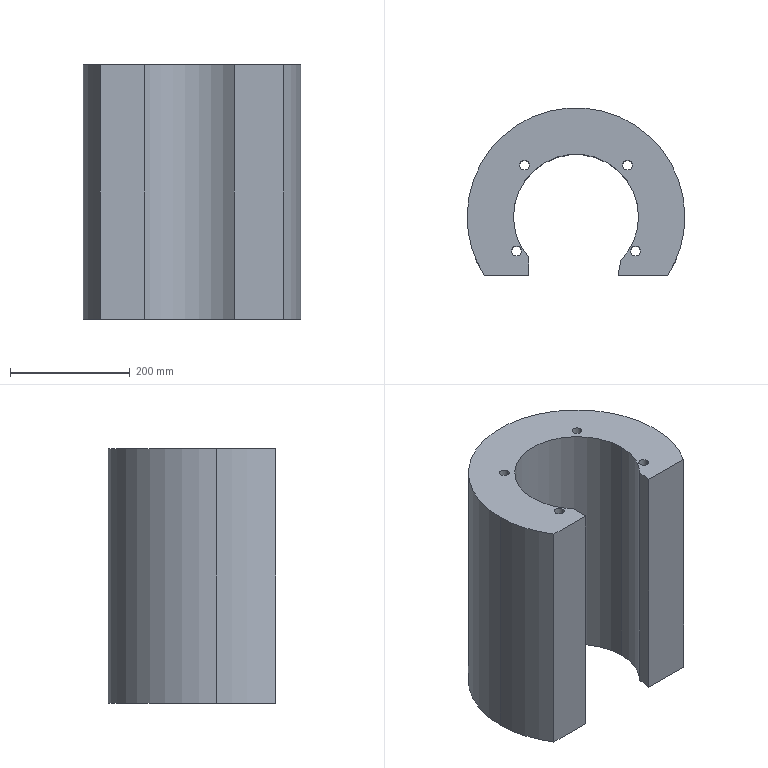Part | SolidWorks | features Extrusion 1 | 1 solid | 20 faces | box 364.306 x 280.408 x 426 mm | volume 21434816 mm3 | cylinder 14 | plane 6 | commonest cylinder face diameters 16 x4 16.5 x4 209.233 x3 364.306 x3
STEP:
#1=CARTESIAN_POINT('',(-19.917,-80.848,-426.));
#2=VERTEX_POINT('',#1);
#3=CARTESIAN_POINT('',(-3.417,-80.848,-426.));
#4=VERTEX_POINT('',#3);
#5=CARTESIAN_POINT('',(-11.667,-80.848,-426.));
#6=DIRECTION('',(0.,0.,1.));
#7=DIRECTION('',(1.,0.,0.));
#8=AXIS2_PLACEMENT_3D('',#5,#6,#7);
#9=CIRCLE('',#8,8.25);
#10=EDGE_CURVE('',#2,#4,#9,.T.);
#11=ORIENTED_EDGE('',*,*,#10,.F.);
#12=CARTESIAN_POINT('',(-19.917,-80.848,0.));
#13=VERTEX_POINT('',#12);
#14=CARTESIAN_POINT('',(-19.917,-80.848,-426.));
#15=DIRECTION('',(0.,0.,1.));
#16=VECTOR('',#15,1000.);
#17=LINE('',#14,#16);
#18=EDGE_CURVE('',#2,#13,#17,.T.);
#19=ORIENTED_EDGE('',*,*,#18,.T.);
#20=CARTESIAN_POINT('',(-3.417,-80.848,0.));
#21=VERTEX_POINT('',#20);
#22=CARTESIAN_POINT('',(-11.667,-80.848,0.));
#23=DIRECTION('',(0.,0.,1.));
#24=DIRECTION('',(1.,0.,0.));
#25=AXIS2_PLACEMENT_3D('',#22,#23,#24);
#26=CIRCLE('',#25,8.25);
#27=EDGE_CURVE('',#13,#21,#26,.T.);
#28=ORIENTED_EDGE('',*,*,#27,.T.);
#29=CARTESIAN_POINT('',(-3.417,-80.848,-426.));
#30=DIRECTION('',(0.,0.,1.));
#31=VECTOR('',#30,1000.);
#32=LINE('',#29,#31);
#33=EDGE_CURVE('',#4,#21,#32,.T.);
#34=ORIENTED_EDGE('',*,*,#33,.F.);
#35=EDGE_LOOP('',(#11,#19,#28,#34));
#36=FACE_OUTER_BOUND('',#35,.T.);
#37=CARTESIAN_POINT('',(-11.667,-80.848,-426.));
#38=DIRECTION('',(0.,0.,1.));
#39=DIRECTION('',(1.,0.,0.));
#40=AXIS2_PLACEMENT_3D('',#37,#38,#39);
#41=CYLINDRICAL_SURFACE('',#40,8.25);
#42=ADVANCED_FACE('',(#36),#41,.F.);
#43=CARTESIAN_POINT('',(-219.103,-80.848,-426.));
#44=VERTEX_POINT('',#43);
#45=CARTESIAN_POINT('',(-202.603,-80.848,-426.));
#46=VERTEX_POINT('',#45);
#47=CARTESIAN_POINT('',(-210.853,-80.848,-426.));
#48=DIRECTION('',(0.,0.,1.));
#49=DIRECTION('',(1.,0.,0.));
#50=AXIS2_PLACEMENT_3D('',#47,#48,#49);
#51=CIRCLE('',#50,8.25);
#52=EDGE_CURVE('',#44,#46,#51,.T.);
#53=ORIENTED_EDGE('',*,*,#52,.F.);
#54=CARTESIAN_POINT('',(-219.103,-80.848,0.));
#55=VERTEX_POINT('',#54);
#56=CARTESIAN_POINT('',(-219.103,-80.848,-426.));
#57=DIRECTION('',(0.,0.,1.));
#58=VECTOR('',#57,1000.);
#59=LINE('',#56,#58);
#60=EDGE_CURVE('',#44,#55,#59,.T.);
#61=ORIENTED_EDGE('',*,*,#60,.T.);
#62=CARTESIAN_POINT('',(-202.603,-80.848,0.));
#63=VERTEX_POINT('',#62);
#64=CARTESIAN_POINT('',(-210.853,-80.848,0.));
#65=DIRECTION('',(0.,0.,1.));
#66=DIRECTION('',(1.,0.,0.));
#67=AXIS2_PLACEMENT_3D('',#64,#65,#66);
#68=CIRCLE('',#67,8.25);
#69=EDGE_CURVE('',#55,#63,#68,.T.);
#70=ORIENTED_EDGE('',*,*,#69,.T.);
#71=CARTESIAN_POINT('',(-202.603,-80.848,-426.));
#72=DIRECTION('',(0.,0.,1.));
#73=VECTOR('',#72,1000.);
#74=LINE('',#71,#73);
#75=EDGE_CURVE('',#46,#63,#74,.T.);
#76=ORIENTED_EDGE('',*,*,#75,.F.);
#77=EDGE_LOOP('',(#53,#61,#70,#76));
#78=FACE_OUTER_BOUND('',#77,.T.);
#79=CARTESIAN_POINT('',(-210.853,-80.848,-426.));
#80=DIRECTION('',(0.,0.,1.));
#81=DIRECTION('',(1.,0.,0.));
#82=AXIS2_PLACEMENT_3D('',#79,#80,#81);
#83=CYLINDRICAL_SURFACE('',#82,8.25);
#84=ADVANCED_FACE('',(#78),#83,.F.);
#85=CARTESIAN_POINT('',(-205.527,62.919,-426.));
#86=VERTEX_POINT('',#85);
#87=CARTESIAN_POINT('',(-189.527,62.919,-426.));
#88=VERTEX_POINT('',#87);
#89=CARTESIAN_POINT('',(-197.527,62.919,-426.));
#90=DIRECTION('',(0.,0.,1.));
#91=DIRECTION('',(1.,0.,0.));
#92=AXIS2_PLACEMENT_3D('',#89,#90,#91);
#93=CIRCLE('',#92,8.);
#94=EDGE_CURVE('',#86,#88,#93,.T.);
#95=ORIENTED_EDGE('',*,*,#94,.F.);
#96=CARTESIAN_POINT('',(-205.527,62.919,0.));
#97=VERTEX_POINT('',#96);
#98=CARTESIAN_POINT('',(-205.527,62.919,-426.));
#99=DIRECTION('',(0.,0.,1.));
#100=VECTOR('',#99,1000.);
#101=LINE('',#98,#100);
#102=EDGE_CURVE('',#86,#97,#101,.T.);
#103=ORIENTED_EDGE('',*,*,#102,.T.);
#104=CARTESIAN_POINT('',(-189.527,62.919,0.));
#105=VERTEX_POINT('',#104);
#106=CARTESIAN_POINT('',(-197.527,62.919,0.));
#107=DIRECTION('',(0.,0.,1.));
#108=DIRECTION('',(1.,0.,0.));
#109=AXIS2_PLACEMENT_3D('',#106,#107,#108);
#110=CIRCLE('',#109,8.);
#111=EDGE_CURVE('',#97,#105,#110,.T.);
#112=ORIENTED_EDGE('',*,*,#111,.T.);
#113=CARTESIAN_POINT('',(-189.527,62.919,-426.));
#114=DIRECTION('',(0.,0.,1.));
#115=VECTOR('',#114,1000.);
#116=LINE('',#113,#115);
#117=EDGE_CURVE('',#88,#105,#116,.T.);
#118=ORIENTED_EDGE('',*,*,#117,.F.);
#119=EDGE_LOOP('',(#95,#103,#112,#118));
#120=FACE_OUTER_BOUND('',#119,.T.);
#121=CARTESIAN_POINT('',(-197.527,62.919,-426.));
#122=DIRECTION('',(0.,0.,1.));
#123=DIRECTION('',(1.,0.,0.));
#124=AXIS2_PLACEMENT_3D('',#121,#122,#123);
#125=CYLINDRICAL_SURFACE('',#124,8.);
#126=ADVANCED_FACE('',(#120),#125,.F.);
#127=CARTESIAN_POINT('',(-32.993,62.919,-426.));
#128=VERTEX_POINT('',#127);
#129=CARTESIAN_POINT('',(-16.993,62.919,-426.));
#130=VERTEX_POINT('',#129);
#131=CARTESIAN_POINT('',(-24.993,62.919,-426.));
#132=DIRECTION('',(0.,0.,1.));
#133=DIRECTION('',(1.,0.,0.));
#134=AXIS2_PLACEMENT_3D('',#131,#132,#133);
#135=CIRCLE('',#134,8.);
#136=EDGE_CURVE('',#128,#130,#135,.T.);
#137=ORIENTED_EDGE('',*,*,#136,.F.);
#138=CARTESIAN_POINT('',(-32.993,62.919,0.));
#139=VERTEX_POINT('',#138);
#140=CARTESIAN_POINT('',(-32.993,62.919,-426.));
#141=DIRECTION('',(0.,0.,1.));
#142=VECTOR('',#141,1000.);
#143=LINE('',#140,#142);
#144=EDGE_CURVE('',#128,#139,#143,.T.);
#145=ORIENTED_EDGE('',*,*,#144,.T.);
#146=CARTESIAN_POINT('',(-16.993,62.919,0.));
#147=VERTEX_POINT('',#146);
#148=CARTESIAN_POINT('',(-24.993,62.919,0.));
#149=DIRECTION('',(0.,0.,1.));
#150=DIRECTION('',(1.,0.,0.));
#151=AXIS2_PLACEMENT_3D('',#148,#149,#150);
#152=CIRCLE('',#151,8.);
#153=EDGE_CURVE('',#139,#147,#152,.T.);
#154=ORIENTED_EDGE('',*,*,#153,.T.);
#155=CARTESIAN_POINT('',(-16.993,62.919,-426.));
#156=DIRECTION('',(0.,0.,1.));
#157=VECTOR('',#156,1000.);
#158=LINE('',#155,#157);
#159=EDGE_CURVE('',#130,#147,#158,.T.);
#160=ORIENTED_EDGE('',*,*,#159,.F.);
#161=EDGE_LOOP('',(#137,#145,#154,#160));
#162=FACE_OUTER_BOUND('',#161,.T.);
#163=CARTESIAN_POINT('',(-24.993,62.919,-426.));
#164=DIRECTION('',(0.,0.,1.));
#165=DIRECTION('',(1.,0.,0.));
#166=AXIS2_PLACEMENT_3D('',#163,#164,#165);
#167=CYLINDRICAL_SURFACE('',#166,8.);
#168=ADVANCED_FACE('',(#162),#167,.F.);
#169=CARTESIAN_POINT('',(-189.998,-92.232,-426.));
#170=VERTEX_POINT('',#169);
#171=CARTESIAN_POINT('',(-215.877,-23.348,-426.));
#172=VERTEX_POINT('',#171);
#173=CARTESIAN_POINT('',(-111.26,-23.348,-426.));
#174=DIRECTION('',(0.,0.,-1.));
#175=DIRECTION('',(1.,0.,0.));
#176=AXIS2_PLACEMENT_3D('',#173,#174,#175);
#177=CIRCLE('',#176,104.617);
#178=EDGE_CURVE('',#170,#172,#177,.T.);
#179=ORIENTED_EDGE('',*,*,#178,.T.);
#180=CARTESIAN_POINT('',(-215.877,-23.348,0.));
#181=VERTEX_POINT('',#180);
#182=CARTESIAN_POINT('',(-215.877,-23.348,-426.));
#183=DIRECTION('',(0.,0.,1.));
#184=VECTOR('',#183,1000.);
#185=LINE('',#182,#184);
#186=EDGE_CURVE('',#172,#181,#185,.T.);
#187=ORIENTED_EDGE('',*,*,#186,.T.);
#188=CARTESIAN_POINT('',(-189.998,-92.232,0.));
#189=VERTEX_POINT('',#188);
#190=CARTESIAN_POINT('',(-111.26,-23.348,0.));
#191=DIRECTION('',(0.,0.,-1.));
#192=DIRECTION('',(1.,0.,0.));
#193=AXIS2_PLACEMENT_3D('',#190,#191,#192);
#194=CIRCLE('',#193,104.617);
#195=EDGE_CURVE('',#189,#181,#194,.T.);
#196=ORIENTED_EDGE('',*,*,#195,.F.);
#197=CARTESIAN_POINT('',(-189.998,-92.232,-426.));
#198=DIRECTION('',(0.,0.,1.));
#199=VECTOR('',#198,1000.);
#200=LINE('',#197,#199);
#201=EDGE_CURVE('',#170,#189,#200,.T.);
#202=ORIENTED_EDGE('',*,*,#201,.F.);
#203=EDGE_LOOP('',(#179,#187,#196,#202));
#204=FACE_OUTER_BOUND('',#203,.T.);
#205=CARTESIAN_POINT('',(-111.26,-23.348,-426.));
#206=DIRECTION('',(0.,0.,1.));
#207=DIRECTION('',(1.,0.,0.));
#208=AXIS2_PLACEMENT_3D('',#205,#206,#207);
#209=CYLINDRICAL_SURFACE('',#208,104.617);
#210=ADVANCED_FACE('',(#204),#209,.F.);
#211=ORIENTED_EDGE('',*,*,#186,.F.);
#212=CARTESIAN_POINT('',(-6.643,-23.348,-426.));
#213=VERTEX_POINT('',#212);
#214=CARTESIAN_POINT('',(-111.26,-23.348,-426.));
#215=DIRECTION('',(0.,0.,-1.));
#216=DIRECTION('',(1.,0.,0.));
#217=AXIS2_PLACEMENT_3D('',#214,#215,#216);
#218=CIRCLE('',#217,104.617);
#219=EDGE_CURVE('',#172,#213,#218,.T.);
#220=ORIENTED_EDGE('',*,*,#219,.T.);
#221=CARTESIAN_POINT('',(-6.643,-23.348,0.));
#222=VERTEX_POINT('',#221);
#223=CARTESIAN_POINT('',(-6.643,-23.348,-426.));
#224=DIRECTION('',(0.,0.,1.));
#225=VECTOR('',#224,1000.);
#226=LINE('',#223,#225);
#227=EDGE_CURVE('',#213,#222,#226,.T.);
#228=ORIENTED_EDGE('',*,*,#227,.T.);
#229=CARTESIAN_POINT('',(-111.26,-23.348,0.));
#230=DIRECTION('',(0.,0.,-1.));
#231=DIRECTION('',(1.,0.,0.));
#232=AXIS2_PLACEMENT_3D('',#229,#230,#231);
#233=CIRCLE('',#232,104.617);
#234=EDGE_CURVE('',#181,#222,#233,.T.);
#235=ORIENTED_EDGE('',*,*,#234,.F.);
#236=EDGE_LOOP('',(#211,#220,#228,#235));
#237=FACE_OUTER_BOUND('',#236,.T.);
#238=CARTESIAN_POINT('',(-111.26,-23.348,-426.));
#239=DIRECTION('',(0.,0.,1.));
#240=DIRECTION('',(1.,0.,0.));
#241=AXIS2_PLACEMENT_3D('',#238,#239,#240);
#242=CYLINDRICAL_SURFACE('',#241,104.617);
#243=ADVANCED_FACE('',(#237),#242,.F.);
#244=CARTESIAN_POINT('',(70.893,-23.348,-426.));
#245=VERTEX_POINT('',#244);
#246=CARTESIAN_POINT('',(-293.413,-23.348,-426.));
#247=VERTEX_POINT('',#246);
#248=CARTESIAN_POINT('',(-111.26,-23.348,-426.));
#249=DIRECTION('',(0.,0.,1.));
#250=DIRECTION('',(1.,0.,0.));
#251=AXIS2_PLACEMENT_3D('',#248,#249,#250);
#252=CIRCLE('',#251,182.153);
#253=EDGE_CURVE('',#245,#247,#252,.T.);
#254=ORIENTED_EDGE('',*,*,#253,.T.);
#255=CARTESIAN_POINT('',(-293.413,-23.348,0.));
#256=VERTEX_POINT('',#255);
#257=CARTESIAN_POINT('',(-293.413,-23.348,-426.));
#258=DIRECTION('',(0.,0.,1.));
#259=VECTOR('',#258,1000.);
#260=LINE('',#257,#259);
#261=EDGE_CURVE('',#247,#256,#260,.T.);
#262=ORIENTED_EDGE('',*,*,#261,.T.);
#263=CARTESIAN_POINT('',(70.893,-23.348,0.));
#264=VERTEX_POINT('',#263);
#265=CARTESIAN_POINT('',(-111.26,-23.348,0.));
#266=DIRECTION('',(0.,0.,1.));
#267=DIRECTION('',(1.,0.,0.));
#268=AXIS2_PLACEMENT_3D('',#265,#266,#267);
#269=CIRCLE('',#268,182.153);
#270=EDGE_CURVE('',#264,#256,#269,.T.);
#271=ORIENTED_EDGE('',*,*,#270,.F.);
#272=CARTESIAN_POINT('',(70.893,-23.348,-426.));
#273=DIRECTION('',(0.,0.,1.));
#274=VECTOR('',#273,1000.);
#275=LINE('',#272,#274);
#276=EDGE_CURVE('',#245,#264,#275,.T.);
#277=ORIENTED_EDGE('',*,*,#276,.F.);
#278=EDGE_LOOP('',(#254,#262,#271,#277));
#279=FACE_OUTER_BOUND('',#278,.T.);
#280=CARTESIAN_POINT('',(-111.26,-23.348,-426.));
#281=DIRECTION('',(0.,0.,1.));
#282=DIRECTION('',(1.,0.,0.));
#283=AXIS2_PLACEMENT_3D('',#280,#281,#282);
#284=CYLINDRICAL_SURFACE('',#283,182.153);
#285=ADVANCED_FACE('',(#279),#284,.T.);
#286=CARTESIAN_POINT('',(42.121,-121.603,-426.));
#287=VERTEX_POINT('',#286);
#288=CARTESIAN_POINT('',(-111.26,-23.348,-426.));
#289=DIRECTION('',(0.,0.,1.));
#290=DIRECTION('',(1.,0.,0.));
#291=AXIS2_PLACEMENT_3D('',#288,#289,#290);
#292=CIRCLE('',#291,182.153);
#293=EDGE_CURVE('',#287,#245,#292,.T.);
#294=ORIENTED_EDGE('',*,*,#293,.T.);
#295=ORIENTED_EDGE('',*,*,#276,.T.);
#296=CARTESIAN_POINT('',(42.121,-121.603,0.));
#297=VERTEX_POINT('',#296);
#298=CARTESIAN_POINT('',(-111.26,-23.348,0.));
#299=DIRECTION('',(0.,0.,1.));
#300=DIRECTION('',(1.,0.,0.));
#301=AXIS2_PLACEMENT_3D('',#298,#299,#300);
#302=CIRCLE('',#301,182.153);
#303=EDGE_CURVE('',#297,#264,#302,.T.);
#304=ORIENTED_EDGE('',*,*,#303,.F.);
#305=CARTESIAN_POINT('',(42.121,-121.603,-426.));
#306=DIRECTION('',(0.,0.,1.));
#307=VECTOR('',#306,1000.);
#308=LINE('',#305,#307);
#309=EDGE_CURVE('',#287,#297,#308,.T.);
#310=ORIENTED_EDGE('',*,*,#309,.F.);
#311=EDGE_LOOP('',(#294,#295,#304,#310));
#312=FACE_OUTER_BOUND('',#311,.T.);
#313=CARTESIAN_POINT('',(-111.26,-23.348,-426.));
#314=DIRECTION('',(0.,0.,1.));
#315=DIRECTION('',(1.,0.,0.));
#316=AXIS2_PLACEMENT_3D('',#313,#314,#315);
#317=CYLINDRICAL_SURFACE('',#316,182.153);
#318=ADVANCED_FACE('',(#312),#317,.T.);
#319=CARTESIAN_POINT('',(-264.641,-121.603,0.));
#320=VERTEX_POINT('',#319);
#321=CARTESIAN_POINT('',(-189.998,-121.603,0.));
#322=VERTEX_POINT('',#321);
#323=CARTESIAN_POINT('',(-189.998,-121.603,0.));
#324=DIRECTION('',(1.,0.,0.));
#325=VECTOR('',#324,1000.);
#326=LINE('',#323,#325);
#327=EDGE_CURVE('',#320,#322,#326,.T.);
#328=ORIENTED_EDGE('',*,*,#327,.F.);
#329=CARTESIAN_POINT('',(-264.641,-121.603,-426.));
#330=VERTEX_POINT('',#329);
#331=CARTESIAN_POINT('',(-264.641,-121.603,-426.));
#332=DIRECTION('',(0.,0.,1.));
#333=VECTOR('',#332,1000.);
#334=LINE('',#331,#333);
#335=EDGE_CURVE('',#330,#320,#334,.T.);
#336=ORIENTED_EDGE('',*,*,#335,.F.);
#337=CARTESIAN_POINT('',(-189.998,-121.603,-426.));
#338=VERTEX_POINT('',#337);
#339=CARTESIAN_POINT('',(-189.998,-121.603,-426.));
#340=DIRECTION('',(1.,0.,0.));
#341=VECTOR('',#340,1000.);
#342=LINE('',#339,#341);
#343=EDGE_CURVE('',#330,#338,#342,.T.);
#344=ORIENTED_EDGE('',*,*,#343,.T.);
#345=CARTESIAN_POINT('',(-189.998,-121.603,-426.));
#346=DIRECTION('',(0.,0.,1.));
#347=VECTOR('',#346,1000.);
#348=LINE('',#345,#347);
#349=EDGE_CURVE('',#338,#322,#348,.T.);
#350=ORIENTED_EDGE('',*,*,#349,.T.);
#351=EDGE_LOOP('',(#328,#336,#344,#350));
#352=FACE_OUTER_BOUND('',#351,.T.);
#353=CARTESIAN_POINT('',(-189.998,-121.603,-426.));
#354=DIRECTION('',(0.,-1.,0.));
#355=DIRECTION('',(0.,0.,-1.));
#356=AXIS2_PLACEMENT_3D('',#353,#354,#355);
#357=PLANE('',#356);
#358=ADVANCED_FACE('',(#352),#357,.T.);
#359=ORIENTED_EDGE('',*,*,#261,.F.);
#360=CARTESIAN_POINT('',(-111.26,-23.348,-426.));
#361=DIRECTION('',(0.,0.,1.));
#362=DIRECTION('',(1.,0.,0.));
#363=AXIS2_PLACEMENT_3D('',#360,#361,#362);
#364=CIRCLE('',#363,182.153);
#365=EDGE_CURVE('',#247,#330,#364,.T.);
#366=ORIENTED_EDGE('',*,*,#365,.T.);
#367=ORIENTED_EDGE('',*,*,#335,.T.);
#368=CARTESIAN_POINT('',(-111.26,-23.348,0.));
#369=DIRECTION('',(0.,0.,1.));
#370=DIRECTION('',(1.,0.,0.));
#371=AXIS2_PLACEMENT_3D('',#368,#369,#370);
#372=CIRCLE('',#371,182.153);
#373=EDGE_CURVE('',#256,#320,#372,.T.);
#374=ORIENTED_EDGE('',*,*,#373,.F.);
#375=EDGE_LOOP('',(#359,#366,#367,#374));
#376=FACE_OUTER_BOUND('',#375,.T.);
#377=CARTESIAN_POINT('',(-111.26,-23.348,-426.));
#378=DIRECTION('',(0.,0.,1.));
#379=DIRECTION('',(1.,0.,0.));
#380=AXIS2_PLACEMENT_3D('',#377,#378,#379);
#381=CYLINDRICAL_SURFACE('',#380,182.153);
#382=ADVANCED_FACE('',(#376),#381,.T.);
#383=CARTESIAN_POINT('',(-40.759,-121.603,0.));
#384=VERTEX_POINT('',#383);
#385=CARTESIAN_POINT('',(42.121,-121.603,0.));
#386=DIRECTION('',(1.,0.,0.));
#387=VECTOR('',#386,1000.);
#388=LINE('',#385,#387);
#389=EDGE_CURVE('',#384,#297,#388,.T.);
#390=ORIENTED_EDGE('',*,*,#389,.F.);
#391=CARTESIAN_POINT('',(-40.759,-121.603,-426.));
#392=VERTEX_POINT('',#391);
#393=CARTESIAN_POINT('',(-40.759,-121.603,-426.));
#394=DIRECTION('',(0.,0.,1.));
#395=VECTOR('',#394,1000.);
#396=LINE('',#393,#395);
#397=EDGE_CURVE('',#392,#384,#396,.T.);
#398=ORIENTED_EDGE('',*,*,#397,.F.);
#399=CARTESIAN_POINT('',(42.121,-121.603,-426.));
#400=DIRECTION('',(1.,0.,0.));
#401=VECTOR('',#400,1000.);
#402=LINE('',#399,#401);
#403=EDGE_CURVE('',#392,#287,#402,.T.);
#404=ORIENTED_EDGE('',*,*,#403,.T.);
#405=ORIENTED_EDGE('',*,*,#309,.T.);
#406=EDGE_LOOP('',(#390,#398,#404,#405));
#407=FACE_OUTER_BOUND('',#406,.T.);
#408=CARTESIAN_POINT('',(42.121,-121.603,-426.));
#409=DIRECTION('',(0.,-1.,0.));
#410=DIRECTION('',(0.,0.,-1.));
#411=AXIS2_PLACEMENT_3D('',#408,#409,#410);
#412=PLANE('',#411);
#413=ADVANCED_FACE('',(#407),#412,.T.);
#414=CARTESIAN_POINT('',(-36.432,-96.46,0.));
#415=VERTEX_POINT('',#414);
#416=CARTESIAN_POINT('',(-40.759,-121.603,0.));
#417=DIRECTION('',(-0.1696,-0.9855,0.));
#418=VECTOR('',#417,1000.);
#419=LINE('',#416,#418);
#420=EDGE_CURVE('',#415,#384,#419,.T.);
#421=ORIENTED_EDGE('',*,*,#420,.F.);
#422=CARTESIAN_POINT('',(-36.432,-96.46,-426.));
#423=VERTEX_POINT('',#422);
#424=CARTESIAN_POINT('',(-36.432,-96.46,-426.));
#425=DIRECTION('',(0.,0.,1.));
#426=VECTOR('',#425,1000.);
#427=LINE('',#424,#426);
#428=EDGE_CURVE('',#423,#415,#427,.T.);
#429=ORIENTED_EDGE('',*,*,#428,.F.);
#430=CARTESIAN_POINT('',(-40.759,-121.603,-426.));
#431=DIRECTION('',(-0.1696,-0.9855,0.));
#432=VECTOR('',#431,1000.);
#433=LINE('',#430,#432);
#434=EDGE_CURVE('',#423,#392,#433,.T.);
#435=ORIENTED_EDGE('',*,*,#434,.T.);
#436=ORIENTED_EDGE('',*,*,#397,.T.);
#437=EDGE_LOOP('',(#421,#429,#435,#436));
#438=FACE_OUTER_BOUND('',#437,.T.);
#439=CARTESIAN_POINT('',(-40.759,-121.603,-426.));
#440=DIRECTION('',(-0.9855,0.1696,0.));
#441=DIRECTION('',(-0.1696,-0.9855,0.));
#442=AXIS2_PLACEMENT_3D('',#439,#440,#441);
#443=PLANE('',#442);
#444=ADVANCED_FACE('',(#438),#443,.T.);
#445=ORIENTED_EDGE('',*,*,#227,.F.);
#446=CARTESIAN_POINT('',(-111.26,-23.348,-426.));
#447=DIRECTION('',(0.,0.,-1.));
#448=DIRECTION('',(1.,0.,0.));
#449=AXIS2_PLACEMENT_3D('',#446,#447,#448);
#450=CIRCLE('',#449,104.617);
#451=EDGE_CURVE('',#213,#423,#450,.T.);
#452=ORIENTED_EDGE('',*,*,#451,.T.);
#453=ORIENTED_EDGE('',*,*,#428,.T.);
#454=CARTESIAN_POINT('',(-111.26,-23.348,0.));
#455=DIRECTION('',(0.,0.,-1.));
#456=DIRECTION('',(1.,0.,0.));
#457=AXIS2_PLACEMENT_3D('',#454,#455,#456);
#458=CIRCLE('',#457,104.617);
#459=EDGE_CURVE('',#222,#415,#458,.T.);
#460=ORIENTED_EDGE('',*,*,#459,.F.);
#461=EDGE_LOOP('',(#445,#452,#453,#460));
#462=FACE_OUTER_BOUND('',#461,.T.);
#463=CARTESIAN_POINT('',(-111.26,-23.348,-426.));
#464=DIRECTION('',(0.,0.,1.));
#465=DIRECTION('',(1.,0.,0.));
#466=AXIS2_PLACEMENT_3D('',#463,#464,#465);
#467=CYLINDRICAL_SURFACE('',#466,104.617);
#468=ADVANCED_FACE('',(#462),#467,.F.);
#469=CARTESIAN_POINT('',(-189.998,-121.603,0.));
#470=DIRECTION('',(0.,1.,0.));
#471=VECTOR('',#470,1000.);
#472=LINE('',#469,#471);
#473=EDGE_CURVE('',#322,#189,#472,.T.);
#474=ORIENTED_EDGE('',*,*,#473,.F.);
#475=ORIENTED_EDGE('',*,*,#349,.F.);
#476=CARTESIAN_POINT('',(-189.998,-121.603,-426.));
#477=DIRECTION('',(0.,1.,0.));
#478=VECTOR('',#477,1000.);
#479=LINE('',#476,#478);
#480=EDGE_CURVE('',#338,#170,#479,.T.);
#481=ORIENTED_EDGE('',*,*,#480,.T.);
#482=ORIENTED_EDGE('',*,*,#201,.T.);
#483=EDGE_LOOP('',(#474,#475,#481,#482));
#484=FACE_OUTER_BOUND('',#483,.T.);
#485=CARTESIAN_POINT('',(-189.998,-121.603,-426.));
#486=DIRECTION('',(1.,0.,0.));
#487=DIRECTION('',(0.,0.,-1.));
#488=AXIS2_PLACEMENT_3D('',#485,#486,#487);
#489=PLANE('',#488);
#490=ADVANCED_FACE('',(#484),#489,.T.);
#491=CARTESIAN_POINT('',(-11.667,-80.848,-426.));
#492=DIRECTION('',(0.,0.,1.));
#493=DIRECTION('',(1.,0.,0.));
#494=AXIS2_PLACEMENT_3D('',#491,#492,#493);
#495=CIRCLE('',#494,8.25);
#496=EDGE_CURVE('',#4,#2,#495,.T.);
#497=ORIENTED_EDGE('',*,*,#496,.T.);
#498=ORIENTED_EDGE('',*,*,#10,.T.);
#499=EDGE_LOOP('',(#497,#498));
#500=FACE_BOUND('',#499,.T.);
#501=CARTESIAN_POINT('',(-210.853,-80.848,-426.));
#502=DIRECTION('',(0.,0.,1.));
#503=DIRECTION('',(1.,0.,0.));
#504=AXIS2_PLACEMENT_3D('',#501,#502,#503);
#505=CIRCLE('',#504,8.25);
#506=EDGE_CURVE('',#46,#44,#505,.T.);
#507=ORIENTED_EDGE('',*,*,#506,.T.);
#508=ORIENTED_EDGE('',*,*,#52,.T.);
#509=EDGE_LOOP('',(#507,#508));
#510=FACE_BOUND('',#509,.T.);
#511=CARTESIAN_POINT('',(-197.527,62.919,-426.));
#512=DIRECTION('',(0.,0.,1.));
#513=DIRECTION('',(1.,0.,0.));
#514=AXIS2_PLACEMENT_3D('',#511,#512,#513);
#515=CIRCLE('',#514,8.);
#516=EDGE_CURVE('',#88,#86,#515,.T.);
#517=ORIENTED_EDGE('',*,*,#516,.T.);
#518=ORIENTED_EDGE('',*,*,#94,.T.);
#519=EDGE_LOOP('',(#517,#518));
#520=FACE_BOUND('',#519,.T.);
#521=CARTESIAN_POINT('',(-24.993,62.919,-426.));
#522=DIRECTION('',(0.,0.,1.));
#523=DIRECTION('',(1.,0.,0.));
#524=AXIS2_PLACEMENT_3D('',#521,#522,#523);
#525=CIRCLE('',#524,8.);
#526=EDGE_CURVE('',#130,#128,#525,.T.);
#527=ORIENTED_EDGE('',*,*,#526,.T.);
#528=ORIENTED_EDGE('',*,*,#136,.T.);
#529=EDGE_LOOP('',(#527,#528));
#530=FACE_BOUND('',#529,.T.);
#531=ORIENTED_EDGE('',*,*,#343,.F.);
#532=ORIENTED_EDGE('',*,*,#365,.F.);
#533=ORIENTED_EDGE('',*,*,#253,.F.);
#534=ORIENTED_EDGE('',*,*,#293,.F.);
#535=ORIENTED_EDGE('',*,*,#403,.F.);
#536=ORIENTED_EDGE('',*,*,#434,.F.);
#537=ORIENTED_EDGE('',*,*,#451,.F.);
#538=ORIENTED_EDGE('',*,*,#219,.F.);
#539=ORIENTED_EDGE('',*,*,#178,.F.);
#540=ORIENTED_EDGE('',*,*,#480,.F.);
#541=EDGE_LOOP('',(#531,#532,#533,#534,#535,#536,#537,#538,#539,#540));
#542=FACE_OUTER_BOUND('',#541,.T.);
#543=CARTESIAN_POINT('',(-111.26,-23.348,-426.));
#544=DIRECTION('',(0.,0.,1.));
#545=DIRECTION('',(1.,0.,0.));
#546=AXIS2_PLACEMENT_3D('',#543,#544,#545);
#547=PLANE('',#546);
#548=ADVANCED_FACE('',(#500,#510,#520,#530,#542),#547,.F.);
#549=CARTESIAN_POINT('',(-11.667,-80.848,0.));
#550=DIRECTION('',(0.,0.,1.));
#551=DIRECTION('',(1.,0.,0.));
#552=AXIS2_PLACEMENT_3D('',#549,#550,#551);
#553=CIRCLE('',#552,8.25);
#554=EDGE_CURVE('',#21,#13,#553,.T.);
#555=ORIENTED_EDGE('',*,*,#554,.F.);
#556=ORIENTED_EDGE('',*,*,#27,.F.);
#557=EDGE_LOOP('',(#555,#556));
#558=FACE_BOUND('',#557,.T.);
#559=CARTESIAN_POINT('',(-210.853,-80.848,0.));
#560=DIRECTION('',(0.,0.,1.));
#561=DIRECTION('',(1.,0.,0.));
#562=AXIS2_PLACEMENT_3D('',#559,#560,#561);
#563=CIRCLE('',#562,8.25);
#564=EDGE_CURVE('',#63,#55,#563,.T.);
#565=ORIENTED_EDGE('',*,*,#564,.F.);
#566=ORIENTED_EDGE('',*,*,#69,.F.);
#567=EDGE_LOOP('',(#565,#566));
#568=FACE_BOUND('',#567,.T.);
#569=CARTESIAN_POINT('',(-197.527,62.919,0.));
#570=DIRECTION('',(0.,0.,1.));
#571=DIRECTION('',(1.,0.,0.));
#572=AXIS2_PLACEMENT_3D('',#569,#570,#571);
#573=CIRCLE('',#572,8.);
#574=EDGE_CURVE('',#105,#97,#573,.T.);
#575=ORIENTED_EDGE('',*,*,#574,.F.);
#576=ORIENTED_EDGE('',*,*,#111,.F.);
#577=EDGE_LOOP('',(#575,#576));
#578=FACE_BOUND('',#577,.T.);
#579=CARTESIAN_POINT('',(-24.993,62.919,0.));
#580=DIRECTION('',(0.,0.,1.));
#581=DIRECTION('',(1.,0.,0.));
#582=AXIS2_PLACEMENT_3D('',#579,#580,#581);
#583=CIRCLE('',#582,8.);
#584=EDGE_CURVE('',#147,#139,#583,.T.);
#585=ORIENTED_EDGE('',*,*,#584,.F.);
#586=ORIENTED_EDGE('',*,*,#153,.F.);
#587=EDGE_LOOP('',(#585,#586));
#588=FACE_BOUND('',#587,.T.);
#589=ORIENTED_EDGE('',*,*,#327,.T.);
#590=ORIENTED_EDGE('',*,*,#473,.T.);
#591=ORIENTED_EDGE('',*,*,#195,.T.);
#592=ORIENTED_EDGE('',*,*,#234,.T.);
#593=ORIENTED_EDGE('',*,*,#459,.T.);
#594=ORIENTED_EDGE('',*,*,#420,.T.);
#595=ORIENTED_EDGE('',*,*,#389,.T.);
#596=ORIENTED_EDGE('',*,*,#303,.T.);
#597=ORIENTED_EDGE('',*,*,#270,.T.);
#598=ORIENTED_EDGE('',*,*,#373,.T.);
#599=EDGE_LOOP('',(#589,#590,#591,#592,#593,#594,#595,#596,#597,#598));
#600=FACE_OUTER_BOUND('',#599,.T.);
#601=CARTESIAN_POINT('',(-111.26,-23.348,0.));
#602=DIRECTION('',(0.,0.,1.));
#603=DIRECTION('',(1.,0.,0.));
#604=AXIS2_PLACEMENT_3D('',#601,#602,#603);
#605=PLANE('',#604);
#606=ADVANCED_FACE('',(#558,#568,#578,#588,#600),#605,.T.);
#607=ORIENTED_EDGE('',*,*,#144,.F.);
#608=ORIENTED_EDGE('',*,*,#526,.F.);
#609=ORIENTED_EDGE('',*,*,#159,.T.);
#610=ORIENTED_EDGE('',*,*,#584,.T.);
#611=EDGE_LOOP('',(#607,#608,#609,#610));
#612=FACE_OUTER_BOUND('',#611,.T.);
#613=CARTESIAN_POINT('',(-24.993,62.919,-426.));
#614=DIRECTION('',(0.,0.,1.));
#615=DIRECTION('',(1.,0.,0.));
#616=AXIS2_PLACEMENT_3D('',#613,#614,#615);
#617=CYLINDRICAL_SURFACE('',#616,8.);
#618=ADVANCED_FACE('',(#612),#617,.F.);
#619=ORIENTED_EDGE('',*,*,#102,.F.);
#620=ORIENTED_EDGE('',*,*,#516,.F.);
#621=ORIENTED_EDGE('',*,*,#117,.T.);
#622=ORIENTED_EDGE('',*,*,#574,.T.);
#623=EDGE_LOOP('',(#619,#620,#621,#622));
#624=FACE_OUTER_BOUND('',#623,.T.);
#625=CARTESIAN_POINT('',(-197.527,62.919,-426.));
#626=DIRECTION('',(0.,0.,1.));
#627=DIRECTION('',(1.,0.,0.));
#628=AXIS2_PLACEMENT_3D('',#625,#626,#627);
#629=CYLINDRICAL_SURFACE('',#628,8.);
#630=ADVANCED_FACE('',(#624),#629,.F.);
#631=ORIENTED_EDGE('',*,*,#60,.F.);
#632=ORIENTED_EDGE('',*,*,#506,.F.);
#633=ORIENTED_EDGE('',*,*,#75,.T.);
#634=ORIENTED_EDGE('',*,*,#564,.T.);
#635=EDGE_LOOP('',(#631,#632,#633,#634));
#636=FACE_OUTER_BOUND('',#635,.T.);
#637=CARTESIAN_POINT('',(-210.853,-80.848,-426.));
#638=DIRECTION('',(0.,0.,1.));
#639=DIRECTION('',(1.,0.,0.));
#640=AXIS2_PLACEMENT_3D('',#637,#638,#639);
#641=CYLINDRICAL_SURFACE('',#640,8.25);
#642=ADVANCED_FACE('',(#636),#641,.F.);
#643=ORIENTED_EDGE('',*,*,#18,.F.);
#644=ORIENTED_EDGE('',*,*,#496,.F.);
#645=ORIENTED_EDGE('',*,*,#33,.T.);
#646=ORIENTED_EDGE('',*,*,#554,.T.);
#647=EDGE_LOOP('',(#643,#644,#645,#646));
#648=FACE_OUTER_BOUND('',#647,.T.);
#649=CARTESIAN_POINT('',(-11.667,-80.848,-426.));
#650=DIRECTION('',(0.,0.,1.));
#651=DIRECTION('',(1.,0.,0.));
#652=AXIS2_PLACEMENT_3D('',#649,#650,#651);
#653=CYLINDRICAL_SURFACE('',#652,8.25);
#654=ADVANCED_FACE('',(#648),#653,.F.);
#655=CLOSED_SHELL('',(#42,#84,#126,#168,#210,#243,#285,#318,#358,#382,#413,#444,#468,#490,#548,#606,#618,#630,#642,#654));
#656=MANIFOLD_SOLID_BREP('',#655);
#657=CARTESIAN_POINT('',(0.,0.,0.));
#658=DIRECTION('',(0.,0.,1.));
#659=DIRECTION('',(1.,0.,0.));
#660=AXIS2_PLACEMENT_3D('',#657,#658,#659);
#661=(LENGTH_UNIT()NAMED_UNIT(*)SI_UNIT(.MILLI.,.METRE.));
#662=UNCERTAINTY_MEASURE_WITH_UNIT(LENGTH_MEASURE(0.00001),#661,'','');
#663=(NAMED_UNIT(*)PLANE_ANGLE_UNIT()SI_UNIT($,.RADIAN.));
#664=(NAMED_UNIT(*)SI_UNIT($,.STERADIAN.)SOLID_ANGLE_UNIT());
#665=(GEOMETRIC_REPRESENTATION_CONTEXT(3)GLOBAL_UNCERTAINTY_ASSIGNED_CONTEXT((#662))GLOBAL_UNIT_ASSIGNED_CONTEXT((#661,#663,#664))REPRESENTATION_CONTEXT('',''));
#666=ADVANCED_BREP_SHAPE_REPRESENTATION('',(#656,#660),#665);